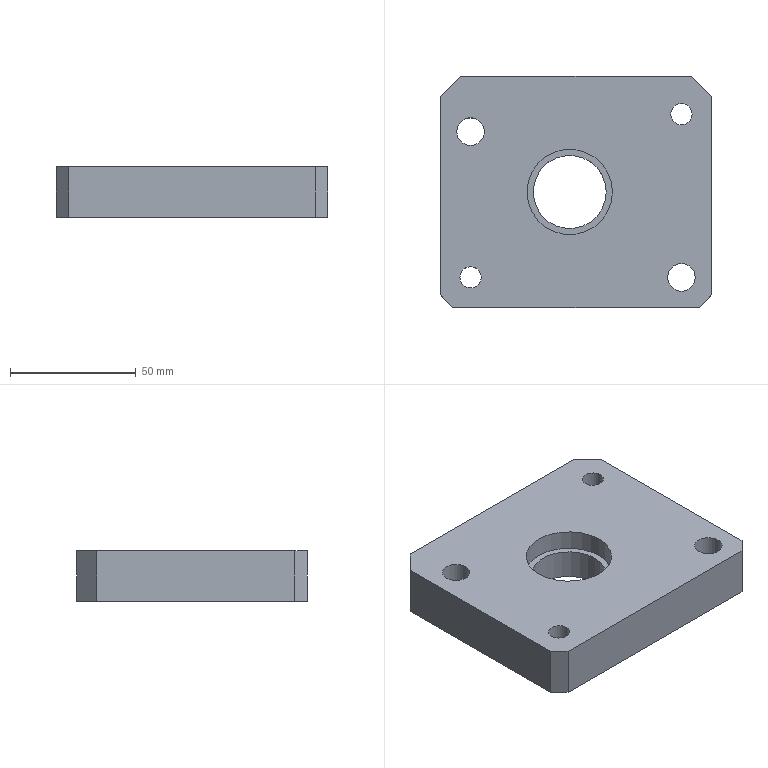Part | STEP file | lll_id3634_x_t | 1 solid | 25 faces | box 108 x 92 x 20 mm | volume 171938 mm3 | plane 15 | cylinder 10 | commonest cylinder face diameters 11 x4 8.5 x2 17 x2 29.07 x1 34 x1
STEP:
#1=CARTESIAN_POINT('',(3325.332,204.288,2.5));
#2=VERTEX_POINT('',#1);
#3=CARTESIAN_POINT('',(3339.867,204.288,2.5));
#4=DIRECTION('',(0.,0.,1.));
#5=DIRECTION('',(-1.,0.,0.));
#6=AXIS2_PLACEMENT_3D('',#3,#4,#5);
#7=CIRCLE('',#6,14.535);
#8=EDGE_CURVE('',#2,#2,#7,.T.);
#9=ORIENTED_EDGE('',*,*,#8,.F.);
#10=EDGE_LOOP('',(#9));
#11=FACE_BOUND('',#10,.T.);
#12=CARTESIAN_POINT('',(3325.332,204.288,14.5));
#13=VERTEX_POINT('',#12);
#14=CARTESIAN_POINT('',(3339.867,204.288,14.5));
#15=DIRECTION('',(0.,0.,1.));
#16=DIRECTION('',(-1.,0.,0.));
#17=AXIS2_PLACEMENT_3D('',#14,#15,#16);
#18=CIRCLE('',#17,14.535);
#19=EDGE_CURVE('',#13,#13,#18,.T.);
#20=ORIENTED_EDGE('',*,*,#19,.T.);
#21=EDGE_LOOP('',(#20));
#22=FACE_BOUND('',#21,.T.);
#23=CARTESIAN_POINT('',(3339.867,204.288,2.5));
#24=DIRECTION('',(0.000000008,0.,-1.));
#25=DIRECTION('',(1.,0.,0.000000008));
#26=AXIS2_PLACEMENT_3D('',#23,#24,#25);
#27=CYLINDRICAL_SURFACE('',#26,14.535);
#28=ADVANCED_FACE('',(#11,#22),#27,.F.);
#29=CARTESIAN_POINT('',(3322.867,204.288,22.5));
#30=VERTEX_POINT('',#29);
#31=CARTESIAN_POINT('',(3339.867,204.288,22.5));
#32=DIRECTION('',(0.,0.,1.));
#33=DIRECTION('',(-1.,0.,0.));
#34=AXIS2_PLACEMENT_3D('',#31,#32,#33);
#35=CIRCLE('',#34,17.);
#36=EDGE_CURVE('',#30,#30,#35,.T.);
#37=ORIENTED_EDGE('',*,*,#36,.F.);
#38=EDGE_LOOP('',(#37));
#39=FACE_BOUND('',#38,.T.);
#40=CARTESIAN_POINT('',(3380.117,235.288,22.5));
#41=VERTEX_POINT('',#40);
#42=CARTESIAN_POINT('',(3384.367,235.288,22.5));
#43=DIRECTION('',(0.,0.,-1.));
#44=DIRECTION('',(-1.,0.,0.));
#45=AXIS2_PLACEMENT_3D('',#42,#43,#44);
#46=CIRCLE('',#45,4.25);
#47=EDGE_CURVE('',#41,#41,#46,.T.);
#48=ORIENTED_EDGE('',*,*,#47,.T.);
#49=EDGE_LOOP('',(#48));
#50=FACE_BOUND('',#49,.T.);
#51=CARTESIAN_POINT('',(3296.117,170.288,22.5));
#52=VERTEX_POINT('',#51);
#53=CARTESIAN_POINT('',(3300.367,170.288,22.5));
#54=DIRECTION('',(0.,0.,-1.));
#55=DIRECTION('',(-1.,0.,0.));
#56=AXIS2_PLACEMENT_3D('',#53,#54,#55);
#57=CIRCLE('',#56,4.25);
#58=EDGE_CURVE('',#52,#52,#57,.T.);
#59=ORIENTED_EDGE('',*,*,#58,.T.);
#60=EDGE_LOOP('',(#59));
#61=FACE_BOUND('',#60,.T.);
#62=CARTESIAN_POINT('',(3378.867,170.288,22.5));
#63=VERTEX_POINT('',#62);
#64=CARTESIAN_POINT('',(3384.367,170.288,22.5));
#65=DIRECTION('',(0.,0.,-1.));
#66=DIRECTION('',(-1.,0.,0.));
#67=AXIS2_PLACEMENT_3D('',#64,#65,#66);
#68=CIRCLE('',#67,5.5);
#69=EDGE_CURVE('',#63,#63,#68,.T.);
#70=ORIENTED_EDGE('',*,*,#69,.T.);
#71=EDGE_LOOP('',(#70));
#72=FACE_BOUND('',#71,.T.);
#73=CARTESIAN_POINT('',(3388.367,250.288,22.5));
#74=VERTEX_POINT('',#73);
#75=CARTESIAN_POINT('',(3296.367,250.288,22.5));
#76=VERTEX_POINT('',#75);
#77=CARTESIAN_POINT('',(3341.867,250.288,22.5));
#78=DIRECTION('',(-1.,0.,0.));
#79=VECTOR('',#78,1.);
#80=LINE('',#77,#79);
#81=EDGE_CURVE('',#74,#76,#80,.T.);
#82=ORIENTED_EDGE('',*,*,#81,.T.);
#83=CARTESIAN_POINT('',(3288.367,242.288,22.5));
#84=VERTEX_POINT('',#83);
#85=CARTESIAN_POINT('',(3431.747,385.668,22.5));
#86=DIRECTION('',(-0.7071,-0.7071,0.));
#87=VECTOR('',#86,1.);
#88=LINE('',#85,#87);
#89=EDGE_CURVE('',#76,#84,#88,.T.);
#90=ORIENTED_EDGE('',*,*,#89,.T.);
#91=CARTESIAN_POINT('',(3288.367,163.288,22.5));
#92=VERTEX_POINT('',#91);
#93=CARTESIAN_POINT('',(3288.367,166.13,22.5));
#94=DIRECTION('',(0.,1.,0.));
#95=VECTOR('',#94,1.);
#96=LINE('',#93,#95);
#97=EDGE_CURVE('',#92,#84,#96,.T.);
#98=ORIENTED_EDGE('',*,*,#97,.F.);
#99=CARTESIAN_POINT('',(3293.367,158.288,22.5));
#100=VERTEX_POINT('',#99);
#101=CARTESIAN_POINT('',(3468.404,-16.749,22.5));
#102=DIRECTION('',(0.7071,-0.7071,0.));
#103=VECTOR('',#102,1.);
#104=LINE('',#101,#103);
#105=EDGE_CURVE('',#92,#100,#104,.T.);
#106=ORIENTED_EDGE('',*,*,#105,.T.);
#107=CARTESIAN_POINT('',(3391.367,158.288,22.5));
#108=VERTEX_POINT('',#107);
#109=CARTESIAN_POINT('',(3341.867,158.288,22.5));
#110=DIRECTION('',(1.,0.,0.));
#111=VECTOR('',#110,1.);
#112=LINE('',#109,#111);
#113=EDGE_CURVE('',#100,#108,#112,.T.);
#114=ORIENTED_EDGE('',*,*,#113,.T.);
#115=CARTESIAN_POINT('',(3396.367,163.288,22.5));
#116=VERTEX_POINT('',#115);
#117=CARTESIAN_POINT('',(3527.747,294.668,22.5));
#118=DIRECTION('',(0.7071,0.7071,0.));
#119=VECTOR('',#118,1.);
#120=LINE('',#117,#119);
#121=EDGE_CURVE('',#108,#116,#120,.T.);
#122=ORIENTED_EDGE('',*,*,#121,.T.);
#123=CARTESIAN_POINT('',(3396.367,242.288,22.5));
#124=VERTEX_POINT('',#123);
#125=CARTESIAN_POINT('',(3396.367,195.288,22.5));
#126=DIRECTION('',(0.,1.,0.));
#127=VECTOR('',#126,1.);
#128=LINE('',#125,#127);
#129=EDGE_CURVE('',#116,#124,#128,.T.);
#130=ORIENTED_EDGE('',*,*,#129,.T.);
#131=CARTESIAN_POINT('',(3564.404,74.251,22.5));
#132=DIRECTION('',(-0.7071,0.7071,0.));
#133=VECTOR('',#132,1.);
#134=LINE('',#131,#133);
#135=EDGE_CURVE('',#124,#74,#134,.T.);
#136=ORIENTED_EDGE('',*,*,#135,.T.);
#137=EDGE_LOOP('',(#82,#90,#98,#106,#114,#122,#130,#136));
#138=FACE_BOUND('',#137,.T.);
#139=CARTESIAN_POINT('',(3294.867,228.288,22.5));
#140=VERTEX_POINT('',#139);
#141=CARTESIAN_POINT('',(3300.367,228.288,22.5));
#142=DIRECTION('',(0.,0.,-1.));
#143=DIRECTION('',(-1.,0.,0.));
#144=AXIS2_PLACEMENT_3D('',#141,#142,#143);
#145=CIRCLE('',#144,5.5);
#146=EDGE_CURVE('',#140,#140,#145,.T.);
#147=ORIENTED_EDGE('',*,*,#146,.T.);
#148=EDGE_LOOP('',(#147));
#149=FACE_BOUND('',#148,.T.);
#150=CARTESIAN_POINT('',(3651.284,166.13,22.5));
#151=DIRECTION('',(0.,0.,1.));
#152=DIRECTION('',(0.,-1.,0.));
#153=AXIS2_PLACEMENT_3D('',#150,#151,#152);
#154=PLANE('',#153);
#155=ADVANCED_FACE('',(#39,#50,#61,#72,#138,#149),#154,.T.);
#156=CARTESIAN_POINT('',(3294.867,170.288,2.5));
#157=VERTEX_POINT('',#156);
#158=CARTESIAN_POINT('',(3300.367,170.288,2.5));
#159=DIRECTION('',(0.,0.,-1.));
#160=DIRECTION('',(-1.,0.,0.));
#161=AXIS2_PLACEMENT_3D('',#158,#159,#160);
#162=CIRCLE('',#161,5.5);
#163=EDGE_CURVE('',#157,#157,#162,.T.);
#164=ORIENTED_EDGE('',*,*,#163,.F.);
#165=EDGE_LOOP('',(#164));
#166=FACE_BOUND('',#165,.T.);
#167=CARTESIAN_POINT('',(3375.867,170.288,2.5));
#168=VERTEX_POINT('',#167);
#169=CARTESIAN_POINT('',(3384.367,170.288,2.5));
#170=DIRECTION('',(0.,0.,1.));
#171=DIRECTION('',(-1.,0.,0.));
#172=AXIS2_PLACEMENT_3D('',#169,#170,#171);
#173=CIRCLE('',#172,8.5);
#174=EDGE_CURVE('',#168,#168,#173,.T.);
#175=ORIENTED_EDGE('',*,*,#174,.T.);
#176=EDGE_LOOP('',(#175));
#177=FACE_BOUND('',#176,.T.);
#178=CARTESIAN_POINT('',(3288.367,242.288,2.5));
#179=VERTEX_POINT('',#178);
#180=CARTESIAN_POINT('',(3288.367,163.288,2.5));
#181=VERTEX_POINT('',#180);
#182=CARTESIAN_POINT('',(3288.367,166.13,2.5));
#183=DIRECTION('',(0.,-1.,0.));
#184=VECTOR('',#183,1.);
#185=LINE('',#182,#184);
#186=EDGE_CURVE('',#179,#181,#185,.T.);
#187=ORIENTED_EDGE('',*,*,#186,.F.);
#188=CARTESIAN_POINT('',(3296.367,250.288,2.5));
#189=VERTEX_POINT('',#188);
#190=CARTESIAN_POINT('',(3431.747,385.668,2.5));
#191=DIRECTION('',(0.7071,0.7071,0.));
#192=VECTOR('',#191,1.);
#193=LINE('',#190,#192);
#194=EDGE_CURVE('',#179,#189,#193,.T.);
#195=ORIENTED_EDGE('',*,*,#194,.T.);
#196=CARTESIAN_POINT('',(3388.367,250.288,2.5));
#197=VERTEX_POINT('',#196);
#198=CARTESIAN_POINT('',(3341.867,250.288,2.5));
#199=DIRECTION('',(1.,0.,0.));
#200=VECTOR('',#199,1.);
#201=LINE('',#198,#200);
#202=EDGE_CURVE('',#189,#197,#201,.T.);
#203=ORIENTED_EDGE('',*,*,#202,.T.);
#204=CARTESIAN_POINT('',(3396.367,242.288,2.5));
#205=VERTEX_POINT('',#204);
#206=CARTESIAN_POINT('',(3564.404,74.251,2.5));
#207=DIRECTION('',(0.7071,-0.7071,0.));
#208=VECTOR('',#207,1.);
#209=LINE('',#206,#208);
#210=EDGE_CURVE('',#197,#205,#209,.T.);
#211=ORIENTED_EDGE('',*,*,#210,.T.);
#212=CARTESIAN_POINT('',(3396.367,163.288,2.5));
#213=VERTEX_POINT('',#212);
#214=CARTESIAN_POINT('',(3396.367,195.288,2.5));
#215=DIRECTION('',(0.,-1.,0.));
#216=VECTOR('',#215,1.);
#217=LINE('',#214,#216);
#218=EDGE_CURVE('',#205,#213,#217,.T.);
#219=ORIENTED_EDGE('',*,*,#218,.T.);
#220=CARTESIAN_POINT('',(3391.367,158.288,2.5));
#221=VERTEX_POINT('',#220);
#222=CARTESIAN_POINT('',(3527.747,294.668,2.5));
#223=DIRECTION('',(-0.7071,-0.7071,0.));
#224=VECTOR('',#223,1.);
#225=LINE('',#222,#224);
#226=EDGE_CURVE('',#213,#221,#225,.T.);
#227=ORIENTED_EDGE('',*,*,#226,.T.);
#228=CARTESIAN_POINT('',(3293.367,158.288,2.5));
#229=VERTEX_POINT('',#228);
#230=CARTESIAN_POINT('',(3341.867,158.288,2.5));
#231=DIRECTION('',(-1.,0.,0.));
#232=VECTOR('',#231,1.);
#233=LINE('',#230,#232);
#234=EDGE_CURVE('',#221,#229,#233,.T.);
#235=ORIENTED_EDGE('',*,*,#234,.T.);
#236=CARTESIAN_POINT('',(3468.404,-16.749,2.5));
#237=DIRECTION('',(-0.7071,0.7071,0.));
#238=VECTOR('',#237,1.);
#239=LINE('',#236,#238);
#240=EDGE_CURVE('',#229,#181,#239,.T.);
#241=ORIENTED_EDGE('',*,*,#240,.T.);
#242=EDGE_LOOP('',(#187,#195,#203,#211,#219,#227,#235,#241));
#243=FACE_BOUND('',#242,.T.);
#244=CARTESIAN_POINT('',(3291.867,228.288,2.5));
#245=VERTEX_POINT('',#244);
#246=CARTESIAN_POINT('',(3300.367,228.288,2.5));
#247=DIRECTION('',(0.,0.,-1.));
#248=DIRECTION('',(-1.,0.,0.));
#249=AXIS2_PLACEMENT_3D('',#246,#247,#248);
#250=CIRCLE('',#249,8.5);
#251=EDGE_CURVE('',#245,#245,#250,.T.);
#252=ORIENTED_EDGE('',*,*,#251,.F.);
#253=EDGE_LOOP('',(#252));
#254=FACE_BOUND('',#253,.T.);
#255=CARTESIAN_POINT('',(3378.867,235.288,2.5));
#256=VERTEX_POINT('',#255);
#257=CARTESIAN_POINT('',(3384.367,235.288,2.5));
#258=DIRECTION('',(0.,0.,1.));
#259=DIRECTION('',(-1.,0.,0.));
#260=AXIS2_PLACEMENT_3D('',#257,#258,#259);
#261=CIRCLE('',#260,5.5);
#262=EDGE_CURVE('',#256,#256,#261,.T.);
#263=ORIENTED_EDGE('',*,*,#262,.T.);
#264=EDGE_LOOP('',(#263));
#265=FACE_BOUND('',#264,.T.);
#266=ORIENTED_EDGE('',*,*,#8,.T.);
#267=EDGE_LOOP('',(#266));
#268=FACE_BOUND('',#267,.T.);
#269=CARTESIAN_POINT('',(3651.284,166.13,2.5));
#270=DIRECTION('',(0.,0.,1.));
#271=DIRECTION('',(0.,-1.,0.));
#272=AXIS2_PLACEMENT_3D('',#269,#270,#271);
#273=PLANE('',#272);
#274=ADVANCED_FACE('',(#166,#177,#243,#254,#265,#268),#273,.F.);
#275=CARTESIAN_POINT('',(3296.117,170.288,9.5));
#276=VERTEX_POINT('',#275);
#277=CARTESIAN_POINT('',(3300.367,170.288,9.5));
#278=DIRECTION('',(0.,0.,1.));
#279=DIRECTION('',(-1.,0.,0.));
#280=AXIS2_PLACEMENT_3D('',#277,#278,#279);
#281=CIRCLE('',#280,4.25);
#282=EDGE_CURVE('',#276,#276,#281,.T.);
#283=ORIENTED_EDGE('',*,*,#282,.T.);
#284=EDGE_LOOP('',(#283));
#285=FACE_BOUND('',#284,.T.);
#286=CARTESIAN_POINT('',(3294.867,170.288,9.5));
#287=VERTEX_POINT('',#286);
#288=CARTESIAN_POINT('',(3300.367,170.288,9.5));
#289=DIRECTION('',(0.,0.,1.));
#290=DIRECTION('',(-1.,0.,0.));
#291=AXIS2_PLACEMENT_3D('',#288,#289,#290);
#292=CIRCLE('',#291,5.5);
#293=EDGE_CURVE('',#287,#287,#292,.T.);
#294=ORIENTED_EDGE('',*,*,#293,.F.);
#295=EDGE_LOOP('',(#294));
#296=FACE_BOUND('',#295,.T.);
#297=CARTESIAN_POINT('',(3300.367,170.288,9.5));
#298=DIRECTION('',(0.,0.,1.));
#299=DIRECTION('',(-1.,0.,0.));
#300=AXIS2_PLACEMENT_3D('',#297,#298,#299);
#301=PLANE('',#300);
#302=ADVANCED_FACE('',(#285,#296),#301,.F.);
#303=CARTESIAN_POINT('',(3378.867,170.288,14.5));
#304=VERTEX_POINT('',#303);
#305=CARTESIAN_POINT('',(3384.367,170.288,14.5));
#306=DIRECTION('',(0.,0.,-1.));
#307=DIRECTION('',(-1.,0.,0.));
#308=AXIS2_PLACEMENT_3D('',#305,#306,#307);
#309=CIRCLE('',#308,5.5);
#310=EDGE_CURVE('',#304,#304,#309,.T.);
#311=ORIENTED_EDGE('',*,*,#310,.F.);
#312=EDGE_LOOP('',(#311));
#313=FACE_BOUND('',#312,.T.);
#314=CARTESIAN_POINT('',(3375.867,170.288,14.5));
#315=VERTEX_POINT('',#314);
#316=CARTESIAN_POINT('',(3384.367,170.288,14.5));
#317=DIRECTION('',(0.,0.,-1.));
#318=DIRECTION('',(-1.,0.,0.));
#319=AXIS2_PLACEMENT_3D('',#316,#317,#318);
#320=CIRCLE('',#319,8.5);
#321=EDGE_CURVE('',#315,#315,#320,.T.);
#322=ORIENTED_EDGE('',*,*,#321,.T.);
#323=EDGE_LOOP('',(#322));
#324=FACE_BOUND('',#323,.T.);
#325=CARTESIAN_POINT('',(3384.367,170.288,14.5));
#326=DIRECTION('',(0.,0.,1.));
#327=DIRECTION('',(0.,1.,0.));
#328=AXIS2_PLACEMENT_3D('',#325,#326,#327);
#329=PLANE('',#328);
#330=ADVANCED_FACE('',(#313,#324),#329,.F.);
#331=CARTESIAN_POINT('',(3294.867,228.288,14.5));
#332=VERTEX_POINT('',#331);
#333=CARTESIAN_POINT('',(3300.367,228.288,14.5));
#334=DIRECTION('',(0.,0.,1.));
#335=DIRECTION('',(-1.,0.,0.));
#336=AXIS2_PLACEMENT_3D('',#333,#334,#335);
#337=CIRCLE('',#336,5.5);
#338=EDGE_CURVE('',#332,#332,#337,.T.);
#339=ORIENTED_EDGE('',*,*,#338,.T.);
#340=EDGE_LOOP('',(#339));
#341=FACE_BOUND('',#340,.T.);
#342=CARTESIAN_POINT('',(3291.867,228.288,14.5));
#343=VERTEX_POINT('',#342);
#344=CARTESIAN_POINT('',(3300.367,228.288,14.5));
#345=DIRECTION('',(0.,0.,1.));
#346=DIRECTION('',(-1.,0.,0.));
#347=AXIS2_PLACEMENT_3D('',#344,#345,#346);
#348=CIRCLE('',#347,8.5);
#349=EDGE_CURVE('',#343,#343,#348,.T.);
#350=ORIENTED_EDGE('',*,*,#349,.F.);
#351=EDGE_LOOP('',(#350));
#352=FACE_BOUND('',#351,.T.);
#353=CARTESIAN_POINT('',(3300.367,228.288,14.5));
#354=DIRECTION('',(0.,0.,1.));
#355=DIRECTION('',(0.,-1.,0.));
#356=AXIS2_PLACEMENT_3D('',#353,#354,#355);
#357=PLANE('',#356);
#358=ADVANCED_FACE('',(#341,#352),#357,.F.);
#359=ORIENTED_EDGE('',*,*,#146,.F.);
#360=EDGE_LOOP('',(#359));
#361=FACE_BOUND('',#360,.T.);
#362=ORIENTED_EDGE('',*,*,#338,.F.);
#363=EDGE_LOOP('',(#362));
#364=FACE_BOUND('',#363,.T.);
#365=CARTESIAN_POINT('',(3300.367,228.288,97.5));
#366=DIRECTION('',(0.,0.,1.));
#367=DIRECTION('',(0.,-1.,0.));
#368=AXIS2_PLACEMENT_3D('',#365,#366,#367);
#369=CYLINDRICAL_SURFACE('',#368,5.5);
#370=ADVANCED_FACE('',(#361,#364),#369,.F.);
#371=ORIENTED_EDGE('',*,*,#293,.T.);
#372=EDGE_LOOP('',(#371));
#373=FACE_BOUND('',#372,.T.);
#374=ORIENTED_EDGE('',*,*,#163,.T.);
#375=EDGE_LOOP('',(#374));
#376=FACE_BOUND('',#375,.T.);
#377=CARTESIAN_POINT('',(3300.367,170.288,-2.5));
#378=DIRECTION('',(0.,0.,1.));
#379=DIRECTION('',(-1.,0.,0.));
#380=AXIS2_PLACEMENT_3D('',#377,#378,#379);
#381=CYLINDRICAL_SURFACE('',#380,5.5);
#382=ADVANCED_FACE('',(#373,#376),#381,.F.);
#383=ORIENTED_EDGE('',*,*,#321,.F.);
#384=EDGE_LOOP('',(#383));
#385=FACE_BOUND('',#384,.T.);
#386=ORIENTED_EDGE('',*,*,#174,.F.);
#387=EDGE_LOOP('',(#386));
#388=FACE_BOUND('',#387,.T.);
#389=CARTESIAN_POINT('',(3384.367,170.288,-2.5));
#390=DIRECTION('',(0.,0.,1.));
#391=DIRECTION('',(0.,1.,0.));
#392=AXIS2_PLACEMENT_3D('',#389,#390,#391);
#393=CYLINDRICAL_SURFACE('',#392,8.5);
#394=ADVANCED_FACE('',(#385,#388),#393,.F.);
#395=ORIENTED_EDGE('',*,*,#218,.F.);
#396=CARTESIAN_POINT('',(3396.367,242.288,-81.5));
#397=DIRECTION('',(0.,0.,1.));
#398=VECTOR('',#397,1.);
#399=LINE('',#396,#398);
#400=EDGE_CURVE('',#205,#124,#399,.T.);
#401=ORIENTED_EDGE('',*,*,#400,.T.);
#402=ORIENTED_EDGE('',*,*,#129,.F.);
#403=CARTESIAN_POINT('',(3396.367,163.288,-81.5));
#404=DIRECTION('',(0.,0.,-1.));
#405=VECTOR('',#404,1.);
#406=LINE('',#403,#405);
#407=EDGE_CURVE('',#116,#213,#406,.T.);
#408=ORIENTED_EDGE('',*,*,#407,.T.);
#409=EDGE_LOOP('',(#395,#401,#402,#408));
#410=FACE_OUTER_BOUND('',#409,.T.);
#411=CARTESIAN_POINT('',(3396.367,195.288,-81.5));
#412=DIRECTION('',(1.,0.,0.));
#413=DIRECTION('',(0.,0.,-1.));
#414=AXIS2_PLACEMENT_3D('',#411,#412,#413);
#415=PLANE('',#414);
#416=ADVANCED_FACE('',(#410),#415,.T.);
#417=ORIENTED_EDGE('',*,*,#234,.F.);
#418=CARTESIAN_POINT('',(3391.367,158.288,-81.5));
#419=DIRECTION('',(0.,0.,1.));
#420=VECTOR('',#419,1.);
#421=LINE('',#418,#420);
#422=EDGE_CURVE('',#221,#108,#421,.T.);
#423=ORIENTED_EDGE('',*,*,#422,.T.);
#424=ORIENTED_EDGE('',*,*,#113,.F.);
#425=CARTESIAN_POINT('',(3293.367,158.288,-81.5));
#426=DIRECTION('',(0.,0.,-1.));
#427=VECTOR('',#426,1.);
#428=LINE('',#425,#427);
#429=EDGE_CURVE('',#100,#229,#428,.T.);
#430=ORIENTED_EDGE('',*,*,#429,.T.);
#431=EDGE_LOOP('',(#417,#423,#424,#430));
#432=FACE_OUTER_BOUND('',#431,.T.);
#433=CARTESIAN_POINT('',(3341.867,158.288,-81.5));
#434=DIRECTION('',(0.,-1.,0.));
#435=DIRECTION('',(0.,0.,-1.));
#436=AXIS2_PLACEMENT_3D('',#433,#434,#435);
#437=PLANE('',#436);
#438=ADVANCED_FACE('',(#432),#437,.T.);
#439=ORIENTED_EDGE('',*,*,#97,.T.);
#440=CARTESIAN_POINT('',(3288.367,242.288,13.5));
#441=DIRECTION('',(0.,0.,-1.));
#442=VECTOR('',#441,1.);
#443=LINE('',#440,#442);
#444=EDGE_CURVE('',#84,#179,#443,.T.);
#445=ORIENTED_EDGE('',*,*,#444,.T.);
#446=ORIENTED_EDGE('',*,*,#186,.T.);
#447=CARTESIAN_POINT('',(3288.367,163.288,13.5));
#448=DIRECTION('',(0.,0.,1.));
#449=VECTOR('',#448,1.);
#450=LINE('',#447,#449);
#451=EDGE_CURVE('',#181,#92,#450,.T.);
#452=ORIENTED_EDGE('',*,*,#451,.T.);
#453=EDGE_LOOP('',(#439,#445,#446,#452));
#454=FACE_OUTER_BOUND('',#453,.T.);
#455=CARTESIAN_POINT('',(3288.367,195.288,13.5));
#456=DIRECTION('',(-1.,0.,0.));
#457=DIRECTION('',(0.,0.,1.));
#458=AXIS2_PLACEMENT_3D('',#455,#456,#457);
#459=PLANE('',#458);
#460=ADVANCED_FACE('',(#454),#459,.T.);
#461=ORIENTED_EDGE('',*,*,#202,.F.);
#462=CARTESIAN_POINT('',(3296.367,250.288,-81.5));
#463=DIRECTION('',(0.,0.,1.));
#464=VECTOR('',#463,1.);
#465=LINE('',#462,#464);
#466=EDGE_CURVE('',#189,#76,#465,.T.);
#467=ORIENTED_EDGE('',*,*,#466,.T.);
#468=ORIENTED_EDGE('',*,*,#81,.F.);
#469=CARTESIAN_POINT('',(3388.367,250.288,-81.5));
#470=DIRECTION('',(0.,0.,-1.));
#471=VECTOR('',#470,1.);
#472=LINE('',#469,#471);
#473=EDGE_CURVE('',#74,#197,#472,.T.);
#474=ORIENTED_EDGE('',*,*,#473,.T.);
#475=EDGE_LOOP('',(#461,#467,#468,#474));
#476=FACE_OUTER_BOUND('',#475,.T.);
#477=CARTESIAN_POINT('',(3341.867,250.288,-81.5));
#478=DIRECTION('',(0.,1.,0.));
#479=DIRECTION('',(0.,0.,1.));
#480=AXIS2_PLACEMENT_3D('',#477,#478,#479);
#481=PLANE('',#480);
#482=ADVANCED_FACE('',(#476),#481,.T.);
#483=ORIENTED_EDGE('',*,*,#349,.T.);
#484=EDGE_LOOP('',(#483));
#485=FACE_BOUND('',#484,.T.);
#486=ORIENTED_EDGE('',*,*,#251,.T.);
#487=EDGE_LOOP('',(#486));
#488=FACE_BOUND('',#487,.T.);
#489=CARTESIAN_POINT('',(3300.367,228.288,-2.5));
#490=DIRECTION('',(0.,0.,1.));
#491=DIRECTION('',(0.,-1.,0.));
#492=AXIS2_PLACEMENT_3D('',#489,#490,#491);
#493=CYLINDRICAL_SURFACE('',#492,8.5);
#494=ADVANCED_FACE('',(#485,#488),#493,.F.);
#495=ORIENTED_EDGE('',*,*,#69,.F.);
#496=EDGE_LOOP('',(#495));
#497=FACE_BOUND('',#496,.T.);
#498=ORIENTED_EDGE('',*,*,#310,.T.);
#499=EDGE_LOOP('',(#498));
#500=FACE_BOUND('',#499,.T.);
#501=CARTESIAN_POINT('',(3384.367,170.288,97.5));
#502=DIRECTION('',(0.,0.,1.));
#503=DIRECTION('',(0.,1.,0.));
#504=AXIS2_PLACEMENT_3D('',#501,#502,#503);
#505=CYLINDRICAL_SURFACE('',#504,5.5);
#506=ADVANCED_FACE('',(#497,#500),#505,.F.);
#507=ORIENTED_EDGE('',*,*,#58,.F.);
#508=EDGE_LOOP('',(#507));
#509=FACE_BOUND('',#508,.T.);
#510=ORIENTED_EDGE('',*,*,#282,.F.);
#511=EDGE_LOOP('',(#510));
#512=FACE_BOUND('',#511,.T.);
#513=CARTESIAN_POINT('',(3300.367,170.288,97.5));
#514=DIRECTION('',(0.,0.,1.));
#515=DIRECTION('',(-1.,0.,0.));
#516=AXIS2_PLACEMENT_3D('',#513,#514,#515);
#517=CYLINDRICAL_SURFACE('',#516,4.25);
#518=ADVANCED_FACE('',(#509,#512),#517,.F.);
#519=ORIENTED_EDGE('',*,*,#47,.F.);
#520=EDGE_LOOP('',(#519));
#521=FACE_BOUND('',#520,.T.);
#522=CARTESIAN_POINT('',(3380.117,235.288,9.5));
#523=VERTEX_POINT('',#522);
#524=CARTESIAN_POINT('',(3384.367,235.288,9.5));
#525=DIRECTION('',(0.,0.,1.));
#526=DIRECTION('',(-1.,0.,0.));
#527=AXIS2_PLACEMENT_3D('',#524,#525,#526);
#528=CIRCLE('',#527,4.25);
#529=EDGE_CURVE('',#523,#523,#528,.T.);
#530=ORIENTED_EDGE('',*,*,#529,.F.);
#531=EDGE_LOOP('',(#530));
#532=FACE_BOUND('',#531,.T.);
#533=CARTESIAN_POINT('',(3384.367,235.288,97.5));
#534=DIRECTION('',(0.,0.,1.));
#535=DIRECTION('',(1.,0.,0.));
#536=AXIS2_PLACEMENT_3D('',#533,#534,#535);
#537=CYLINDRICAL_SURFACE('',#536,4.25);
#538=ADVANCED_FACE('',(#521,#532),#537,.F.);
#539=ORIENTED_EDGE('',*,*,#529,.T.);
#540=EDGE_LOOP('',(#539));
#541=FACE_BOUND('',#540,.T.);
#542=CARTESIAN_POINT('',(3378.867,235.288,9.5));
#543=VERTEX_POINT('',#542);
#544=CARTESIAN_POINT('',(3384.367,235.288,9.5));
#545=DIRECTION('',(0.,0.,1.));
#546=DIRECTION('',(-1.,0.,0.));
#547=AXIS2_PLACEMENT_3D('',#544,#545,#546);
#548=CIRCLE('',#547,5.5);
#549=EDGE_CURVE('',#543,#543,#548,.T.);
#550=ORIENTED_EDGE('',*,*,#549,.F.);
#551=EDGE_LOOP('',(#550));
#552=FACE_BOUND('',#551,.T.);
#553=CARTESIAN_POINT('',(3384.367,235.288,9.5));
#554=DIRECTION('',(0.,0.,1.));
#555=DIRECTION('',(1.,0.,0.));
#556=AXIS2_PLACEMENT_3D('',#553,#554,#555);
#557=PLANE('',#556);
#558=ADVANCED_FACE('',(#541,#552),#557,.F.);
#559=ORIENTED_EDGE('',*,*,#549,.T.);
#560=EDGE_LOOP('',(#559));
#561=FACE_BOUND('',#560,.T.);
#562=ORIENTED_EDGE('',*,*,#262,.F.);
#563=EDGE_LOOP('',(#562));
#564=FACE_BOUND('',#563,.T.);
#565=CARTESIAN_POINT('',(3384.367,235.288,-2.5));
#566=DIRECTION('',(0.,0.,1.));
#567=DIRECTION('',(1.,0.,0.));
#568=AXIS2_PLACEMENT_3D('',#565,#566,#567);
#569=CYLINDRICAL_SURFACE('',#568,5.5);
#570=ADVANCED_FACE('',(#561,#564),#569,.F.);
#571=ORIENTED_EDGE('',*,*,#36,.T.);
#572=EDGE_LOOP('',(#571));
#573=FACE_BOUND('',#572,.T.);
#574=CARTESIAN_POINT('',(3322.867,204.288,14.5));
#575=VERTEX_POINT('',#574);
#576=CARTESIAN_POINT('',(3339.867,204.288,14.5));
#577=DIRECTION('',(0.,0.,-1.));
#578=DIRECTION('',(-1.,0.,0.));
#579=AXIS2_PLACEMENT_3D('',#576,#577,#578);
#580=CIRCLE('',#579,17.);
#581=EDGE_CURVE('',#575,#575,#580,.T.);
#582=ORIENTED_EDGE('',*,*,#581,.T.);
#583=EDGE_LOOP('',(#582));
#584=FACE_BOUND('',#583,.T.);
#585=CARTESIAN_POINT('',(3339.867,204.288,14.5));
#586=DIRECTION('',(0.,0.,1.));
#587=DIRECTION('',(-1.,0.,0.));
#588=AXIS2_PLACEMENT_3D('',#585,#586,#587);
#589=CYLINDRICAL_SURFACE('',#588,17.);
#590=ADVANCED_FACE('',(#573,#584),#589,.F.);
#591=ORIENTED_EDGE('',*,*,#19,.F.);
#592=EDGE_LOOP('',(#591));
#593=FACE_BOUND('',#592,.T.);
#594=ORIENTED_EDGE('',*,*,#581,.F.);
#595=EDGE_LOOP('',(#594));
#596=FACE_BOUND('',#595,.T.);
#597=CARTESIAN_POINT('',(3339.867,204.288,14.5));
#598=DIRECTION('',(0.,0.,1.));
#599=DIRECTION('',(-1.,0.,0.));
#600=AXIS2_PLACEMENT_3D('',#597,#598,#599);
#601=PLANE('',#600);
#602=ADVANCED_FACE('',(#593,#596),#601,.T.);
#603=ORIENTED_EDGE('',*,*,#121,.F.);
#604=ORIENTED_EDGE('',*,*,#422,.F.);
#605=ORIENTED_EDGE('',*,*,#226,.F.);
#606=ORIENTED_EDGE('',*,*,#407,.F.);
#607=EDGE_LOOP('',(#603,#604,#605,#606));
#608=FACE_OUTER_BOUND('',#607,.T.);
#609=CARTESIAN_POINT('',(3396.367,163.288,-81.5));
#610=DIRECTION('',(-0.7071,0.7071,0.));
#611=DIRECTION('',(0.,0.,-1.));
#612=AXIS2_PLACEMENT_3D('',#609,#610,#611);
#613=PLANE('',#612);
#614=ADVANCED_FACE('',(#608),#613,.F.);
#615=ORIENTED_EDGE('',*,*,#105,.F.);
#616=ORIENTED_EDGE('',*,*,#451,.F.);
#617=ORIENTED_EDGE('',*,*,#240,.F.);
#618=ORIENTED_EDGE('',*,*,#429,.F.);
#619=EDGE_LOOP('',(#615,#616,#617,#618));
#620=FACE_OUTER_BOUND('',#619,.T.);
#621=CARTESIAN_POINT('',(3293.367,158.288,-81.5));
#622=DIRECTION('',(0.7071,0.7071,0.));
#623=DIRECTION('',(0.,0.,-1.));
#624=AXIS2_PLACEMENT_3D('',#621,#622,#623);
#625=PLANE('',#624);
#626=ADVANCED_FACE('',(#620),#625,.F.);
#627=ORIENTED_EDGE('',*,*,#194,.F.);
#628=ORIENTED_EDGE('',*,*,#444,.F.);
#629=ORIENTED_EDGE('',*,*,#89,.F.);
#630=ORIENTED_EDGE('',*,*,#466,.F.);
#631=EDGE_LOOP('',(#627,#628,#629,#630));
#632=FACE_OUTER_BOUND('',#631,.T.);
#633=CARTESIAN_POINT('',(3296.367,250.288,-81.5));
#634=DIRECTION('',(0.7071,-0.7071,0.));
#635=DIRECTION('',(0.,0.,1.));
#636=AXIS2_PLACEMENT_3D('',#633,#634,#635);
#637=PLANE('',#636);
#638=ADVANCED_FACE('',(#632),#637,.F.);
#639=ORIENTED_EDGE('',*,*,#135,.F.);
#640=ORIENTED_EDGE('',*,*,#400,.F.);
#641=ORIENTED_EDGE('',*,*,#210,.F.);
#642=ORIENTED_EDGE('',*,*,#473,.F.);
#643=EDGE_LOOP('',(#639,#640,#641,#642));
#644=FACE_OUTER_BOUND('',#643,.T.);
#645=CARTESIAN_POINT('',(3388.367,250.288,-81.5));
#646=DIRECTION('',(-0.7071,-0.7071,0.));
#647=DIRECTION('',(0.,0.,-1.));
#648=AXIS2_PLACEMENT_3D('',#645,#646,#647);
#649=PLANE('',#648);
#650=ADVANCED_FACE('',(#644),#649,.F.);
#651=CLOSED_SHELL('',(#28,#155,#274,#302,#330,#358,#370,#382,#394,#416,#438,#460,#482,#494,#506,#518,#538,#558,#570,#590,#602,#614,#626,#638,#650));
#652=MANIFOLD_SOLID_BREP('',#651);
#653=(LENGTH_UNIT()NAMED_UNIT(*)SI_UNIT(.MILLI.,.METRE.));
#654=UNCERTAINTY_MEASURE_WITH_UNIT(LENGTH_MEASURE(0.00002),#653,'','');
#655=(NAMED_UNIT(*)PLANE_ANGLE_UNIT()SI_UNIT($,.RADIAN.));
#656=PLANE_ANGLE_MEASURE_WITH_UNIT(PLANE_ANGLE_MEASURE(0.01745),#655);
#657=DIMENSIONAL_EXPONENTS(0.,0.,0.,0.,0.,0.,0.);
#658=(CONVERSION_BASED_UNIT('DEGREE',#656)NAMED_UNIT(#657)PLANE_ANGLE_UNIT());
#659=(NAMED_UNIT(*)SI_UNIT($,.STERADIAN.)SOLID_ANGLE_UNIT());
#660=(GEOMETRIC_REPRESENTATION_CONTEXT(3)GLOBAL_UNCERTAINTY_ASSIGNED_CONTEXT((#654))GLOBAL_UNIT_ASSIGNED_CONTEXT((#653,#658,#659))REPRESENTATION_CONTEXT('',''));
#661=ADVANCED_BREP_SHAPE_REPRESENTATION('',(#652),#660);